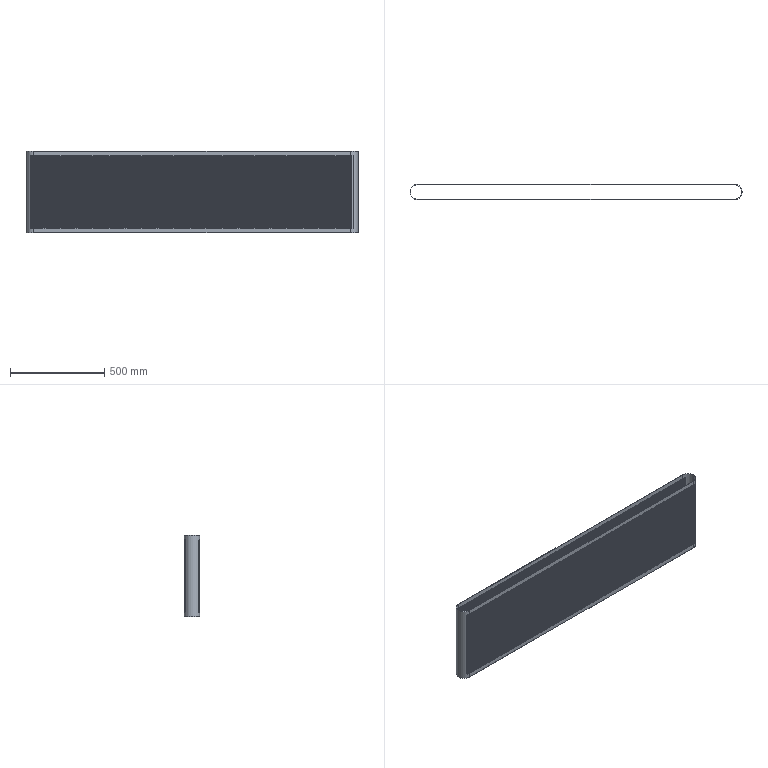Part | STEP file | 1 solid | 1732 faces | box 1763 x 82 x 434 mm | volume 1814355 mm3 | cylinder 1038 | plane 694 | commonest cylinder face diameters 5 x1032 78 x3 82 x3